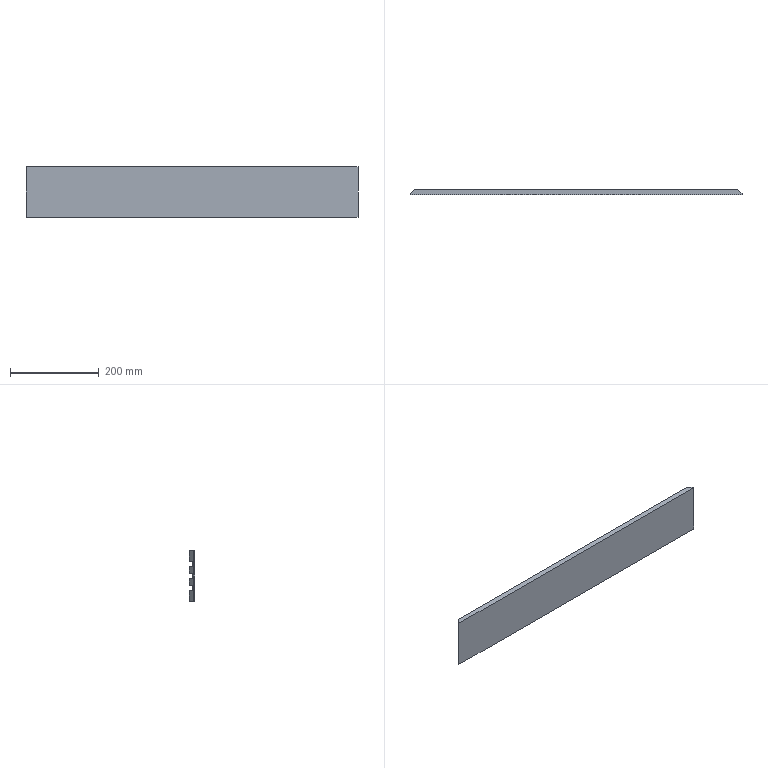Part | STEP file | 012-6-07-08 | 1 solid | 20 faces | box 750 x 12 x 114 mm | volume 828876 mm3 | plane 20
STEP:
#1=CARTESIAN_POINT('',(0.,0.,0.));
#2=DIRECTION('',(0.,0.,1.));
#3=DIRECTION('',(1.,0.,0.));
#4=AXIS2_PLACEMENT_3D('',#1,#2,#3);
#5=CARTESIAN_POINT('',(365.,6.,78.5));
#6=VERTEX_POINT('',#5);
#7=CARTESIAN_POINT('',(365.,6.,63.));
#8=VERTEX_POINT('',#7);
#9=CARTESIAN_POINT('',(365.,6.,114.));
#10=DIRECTION('',(0.,0.,-1.));
#11=VECTOR('',#10,1.);
#12=LINE('',#9,#11);
#13=CARTESIAN_POINT('',(-375.,6.,114.));
#14=DIRECTION('',(0.,-1.,0.));
#15=DIRECTION('',(0.,0.,-1.));
#16=AXIS2_PLACEMENT_3D('',#13,#14,#15);
#17=PLANE('',#16);
#18=CARTESIAN_POINT('',(0.,740.));
#19=DIRECTION('',(1.,0.));
#20=VECTOR('',#19,1.);
#21=LINE('',#18,#20);
#22=(GEOMETRIC_REPRESENTATION_CONTEXT(2)PARAMETRIC_REPRESENTATION_CONTEXT()REPRESENTATION_CONTEXT('',''));
#23=DEFINITIONAL_REPRESENTATION('',(#21),#22);
#24=PCURVE('',#17,#23);
#25=CARTESIAN_POINT('',(365.,6.,114.));
#26=DIRECTION('',(-0.7071,-0.7071,0.));
#27=DIRECTION('',(0.7071,-0.7071,0.));
#28=AXIS2_PLACEMENT_3D('',#25,#26,#27);
#29=PLANE('',#28);
#30=CARTESIAN_POINT('',(0.,0.));
#31=DIRECTION('',(0.,-1.));
#32=VECTOR('',#31,1.);
#33=LINE('',#30,#32);
#34=(GEOMETRIC_REPRESENTATION_CONTEXT(2)PARAMETRIC_REPRESENTATION_CONTEXT()REPRESENTATION_CONTEXT('',''));
#35=DEFINITIONAL_REPRESENTATION('',(#33),#34);
#36=PCURVE('',#29,#35);
#37=SURFACE_CURVE('',#12,(#24,#36),.PCURVE_S1.);
#38=EDGE_CURVE('',#6,#8,#37,.T.);
#39=ORIENTED_EDGE('',*,*,#38,.T.);
#40=CARTESIAN_POINT('',(-365.,6.,63.));
#41=VERTEX_POINT('',#40);
#42=CARTESIAN_POINT('',(378.993,6.,63.));
#43=DIRECTION('',(1.,0.,0.));
#44=VECTOR('',#43,1.);
#45=LINE('',#42,#44);
#46=CARTESIAN_POINT('',(51.,753.993));
#47=DIRECTION('',(0.,1.));
#48=VECTOR('',#47,1.);
#49=LINE('',#46,#48);
#50=(GEOMETRIC_REPRESENTATION_CONTEXT(2)PARAMETRIC_REPRESENTATION_CONTEXT()REPRESENTATION_CONTEXT('',''));
#51=DEFINITIONAL_REPRESENTATION('',(#49),#50);
#52=PCURVE('',#17,#51);
#53=CARTESIAN_POINT('',(378.993,-1.,63.));
#54=DIRECTION('',(0.,0.,1.));
#55=DIRECTION('',(1.,0.,0.));
#56=AXIS2_PLACEMENT_3D('',#53,#54,#55);
#57=PLANE('',#56);
#58=CARTESIAN_POINT('',(0.,7.));
#59=DIRECTION('',(1.,0.));
#60=VECTOR('',#59,1.);
#61=LINE('',#58,#60);
#62=(GEOMETRIC_REPRESENTATION_CONTEXT(2)PARAMETRIC_REPRESENTATION_CONTEXT()REPRESENTATION_CONTEXT('',''));
#63=DEFINITIONAL_REPRESENTATION('',(#61),#62);
#64=PCURVE('',#57,#63);
#65=SURFACE_CURVE('',#45,(#52,#64),.PCURVE_S1.);
#66=EDGE_CURVE('',#41,#8,#65,.T.);
#67=ORIENTED_EDGE('',*,*,#66,.F.);
#68=CARTESIAN_POINT('',(-365.,6.,78.5));
#69=VERTEX_POINT('',#68);
#70=CARTESIAN_POINT('',(-365.,6.,114.));
#71=DIRECTION('',(0.,0.,1.));
#72=VECTOR('',#71,1.);
#73=LINE('',#70,#72);
#74=CARTESIAN_POINT('',(0.,10.));
#75=DIRECTION('',(-1.,0.));
#76=VECTOR('',#75,1.);
#77=LINE('',#74,#76);
#78=(GEOMETRIC_REPRESENTATION_CONTEXT(2)PARAMETRIC_REPRESENTATION_CONTEXT()REPRESENTATION_CONTEXT('',''));
#79=DEFINITIONAL_REPRESENTATION('',(#77),#78);
#80=PCURVE('',#17,#79);
#81=CARTESIAN_POINT('',(-375.,-4.,114.));
#82=DIRECTION('',(0.7071,-0.7071,0.));
#83=DIRECTION('',(0.7071,0.7071,0.));
#84=AXIS2_PLACEMENT_3D('',#81,#82,#83);
#85=PLANE('',#84);
#86=CARTESIAN_POINT('',(14.142,0.));
#87=DIRECTION('',(0.,1.));
#88=VECTOR('',#87,1.);
#89=LINE('',#86,#88);
#90=(GEOMETRIC_REPRESENTATION_CONTEXT(2)PARAMETRIC_REPRESENTATION_CONTEXT()REPRESENTATION_CONTEXT('',''));
#91=DEFINITIONAL_REPRESENTATION('',(#89),#90);
#92=PCURVE('',#85,#91);
#93=SURFACE_CURVE('',#73,(#80,#92),.PCURVE_S1.);
#94=EDGE_CURVE('',#41,#69,#93,.T.);
#95=ORIENTED_EDGE('',*,*,#94,.T.);
#96=CARTESIAN_POINT('',(378.993,6.,78.5));
#97=DIRECTION('',(-1.,0.,0.));
#98=VECTOR('',#97,1.);
#99=LINE('',#96,#98);
#100=CARTESIAN_POINT('',(35.5,753.993));
#101=DIRECTION('',(0.,-1.));
#102=VECTOR('',#101,1.);
#103=LINE('',#100,#102);
#104=(GEOMETRIC_REPRESENTATION_CONTEXT(2)PARAMETRIC_REPRESENTATION_CONTEXT()REPRESENTATION_CONTEXT('',''));
#105=DEFINITIONAL_REPRESENTATION('',(#103),#104);
#106=PCURVE('',#17,#105);
#107=CARTESIAN_POINT('',(378.993,-1.,78.5));
#108=DIRECTION('',(0.,0.,-1.));
#109=DIRECTION('',(-1.,0.,0.));
#110=AXIS2_PLACEMENT_3D('',#107,#108,#109);
#111=PLANE('',#110);
#112=CARTESIAN_POINT('',(0.,7.));
#113=DIRECTION('',(1.,0.));
#114=VECTOR('',#113,1.);
#115=LINE('',#112,#114);
#116=(GEOMETRIC_REPRESENTATION_CONTEXT(2)PARAMETRIC_REPRESENTATION_CONTEXT()REPRESENTATION_CONTEXT('',''));
#117=DEFINITIONAL_REPRESENTATION('',(#115),#116);
#118=PCURVE('',#111,#117);
#119=SURFACE_CURVE('',#99,(#106,#118),.PCURVE_S1.);
#120=EDGE_CURVE('',#6,#69,#119,.T.);
#121=ORIENTED_EDGE('',*,*,#120,.F.);
#122=EDGE_LOOP('',(#39,#67,#95,#121));
#123=FACE_BOUND('',#122,.T.);
#124=ADVANCED_FACE('',(#123),#17,.F.);
#125=CARTESIAN_POINT('',(365.,6.,114.));
#126=VERTEX_POINT('',#125);
#127=CARTESIAN_POINT('',(365.,6.,90.5));
#128=VERTEX_POINT('',#127);
#129=CARTESIAN_POINT('',(365.,6.,114.));
#130=DIRECTION('',(0.,0.,-1.));
#131=VECTOR('',#130,1.);
#132=LINE('',#129,#131);
#133=CARTESIAN_POINT('',(-375.,6.,114.));
#134=DIRECTION('',(0.,-1.,0.));
#135=DIRECTION('',(0.,0.,-1.));
#136=AXIS2_PLACEMENT_3D('',#133,#134,#135);
#137=PLANE('',#136);
#138=CARTESIAN_POINT('',(0.,740.));
#139=DIRECTION('',(1.,0.));
#140=VECTOR('',#139,1.);
#141=LINE('',#138,#140);
#142=(GEOMETRIC_REPRESENTATION_CONTEXT(2)PARAMETRIC_REPRESENTATION_CONTEXT()REPRESENTATION_CONTEXT('',''));
#143=DEFINITIONAL_REPRESENTATION('',(#141),#142);
#144=PCURVE('',#137,#143);
#145=CARTESIAN_POINT('',(0.,0.));
#146=DIRECTION('',(0.,-1.));
#147=VECTOR('',#146,1.);
#148=LINE('',#145,#147);
#149=(GEOMETRIC_REPRESENTATION_CONTEXT(2)PARAMETRIC_REPRESENTATION_CONTEXT()REPRESENTATION_CONTEXT('',''));
#150=DEFINITIONAL_REPRESENTATION('',(#148),#149);
#151=PCURVE('',#29,#150);
#152=SURFACE_CURVE('',#132,(#144,#151),.PCURVE_S1.);
#153=EDGE_CURVE('',#126,#128,#152,.T.);
#154=ORIENTED_EDGE('',*,*,#153,.T.);
#155=CARTESIAN_POINT('',(-365.,6.,90.5));
#156=VERTEX_POINT('',#155);
#157=CARTESIAN_POINT('',(378.993,6.,90.5));
#158=DIRECTION('',(1.,0.,0.));
#159=VECTOR('',#158,1.);
#160=LINE('',#157,#159);
#161=CARTESIAN_POINT('',(23.5,753.993));
#162=DIRECTION('',(0.,1.));
#163=VECTOR('',#162,1.);
#164=LINE('',#161,#163);
#165=(GEOMETRIC_REPRESENTATION_CONTEXT(2)PARAMETRIC_REPRESENTATION_CONTEXT()REPRESENTATION_CONTEXT('',''));
#166=DEFINITIONAL_REPRESENTATION('',(#164),#165);
#167=PCURVE('',#137,#166);
#168=CARTESIAN_POINT('',(378.993,-1.,90.5));
#169=DIRECTION('',(0.,0.,1.));
#170=DIRECTION('',(1.,0.,0.));
#171=AXIS2_PLACEMENT_3D('',#168,#169,#170);
#172=PLANE('',#171);
#173=CARTESIAN_POINT('',(0.,7.));
#174=DIRECTION('',(1.,0.));
#175=VECTOR('',#174,1.);
#176=LINE('',#173,#175);
#177=(GEOMETRIC_REPRESENTATION_CONTEXT(2)PARAMETRIC_REPRESENTATION_CONTEXT()REPRESENTATION_CONTEXT('',''));
#178=DEFINITIONAL_REPRESENTATION('',(#176),#177);
#179=PCURVE('',#172,#178);
#180=SURFACE_CURVE('',#160,(#167,#179),.PCURVE_S1.);
#181=EDGE_CURVE('',#156,#128,#180,.T.);
#182=ORIENTED_EDGE('',*,*,#181,.F.);
#183=CARTESIAN_POINT('',(-365.,6.,114.));
#184=VERTEX_POINT('',#183);
#185=CARTESIAN_POINT('',(-365.,6.,114.));
#186=DIRECTION('',(0.,0.,1.));
#187=VECTOR('',#186,1.);
#188=LINE('',#185,#187);
#189=CARTESIAN_POINT('',(0.,10.));
#190=DIRECTION('',(-1.,0.));
#191=VECTOR('',#190,1.);
#192=LINE('',#189,#191);
#193=(GEOMETRIC_REPRESENTATION_CONTEXT(2)PARAMETRIC_REPRESENTATION_CONTEXT()REPRESENTATION_CONTEXT('',''));
#194=DEFINITIONAL_REPRESENTATION('',(#192),#193);
#195=PCURVE('',#137,#194);
#196=CARTESIAN_POINT('',(14.142,0.));
#197=DIRECTION('',(0.,1.));
#198=VECTOR('',#197,1.);
#199=LINE('',#196,#198);
#200=(GEOMETRIC_REPRESENTATION_CONTEXT(2)PARAMETRIC_REPRESENTATION_CONTEXT()REPRESENTATION_CONTEXT('',''));
#201=DEFINITIONAL_REPRESENTATION('',(#199),#200);
#202=PCURVE('',#85,#201);
#203=SURFACE_CURVE('',#188,(#195,#202),.PCURVE_S1.);
#204=EDGE_CURVE('',#156,#184,#203,.T.);
#205=ORIENTED_EDGE('',*,*,#204,.T.);
#206=CARTESIAN_POINT('',(-375.,6.,114.));
#207=DIRECTION('',(-1.,0.,0.));
#208=VECTOR('',#207,1.);
#209=LINE('',#206,#208);
#210=CARTESIAN_POINT('',(0.,0.));
#211=DIRECTION('',(0.,-1.));
#212=VECTOR('',#211,1.);
#213=LINE('',#210,#212);
#214=(GEOMETRIC_REPRESENTATION_CONTEXT(2)PARAMETRIC_REPRESENTATION_CONTEXT()REPRESENTATION_CONTEXT('',''));
#215=DEFINITIONAL_REPRESENTATION('',(#213),#214);
#216=PCURVE('',#137,#215);
#217=CARTESIAN_POINT('',(375.,-6.,114.));
#218=DIRECTION('',(0.,0.,1.));
#219=DIRECTION('',(1.,0.,0.));
#220=AXIS2_PLACEMENT_3D('',#217,#218,#219);
#221=PLANE('',#220);
#222=CARTESIAN_POINT('',(-750.,12.));
#223=DIRECTION('',(-1.,0.));
#224=VECTOR('',#223,1.);
#225=LINE('',#222,#224);
#226=(GEOMETRIC_REPRESENTATION_CONTEXT(2)PARAMETRIC_REPRESENTATION_CONTEXT()REPRESENTATION_CONTEXT('',''));
#227=DEFINITIONAL_REPRESENTATION('',(#225),#226);
#228=PCURVE('',#221,#227);
#229=SURFACE_CURVE('',#209,(#216,#228),.PCURVE_S1.);
#230=EDGE_CURVE('',#126,#184,#229,.T.);
#231=ORIENTED_EDGE('',*,*,#230,.F.);
#232=EDGE_LOOP('',(#154,#182,#205,#231));
#233=FACE_BOUND('',#232,.T.);
#234=ADVANCED_FACE('',(#233),#137,.F.);
#235=CARTESIAN_POINT('',(-365.,6.,35.5));
#236=VERTEX_POINT('',#235);
#237=CARTESIAN_POINT('',(-365.,6.,51.));
#238=VERTEX_POINT('',#237);
#239=CARTESIAN_POINT('',(-365.,6.,114.));
#240=DIRECTION('',(0.,0.,1.));
#241=VECTOR('',#240,1.);
#242=LINE('',#239,#241);
#243=CARTESIAN_POINT('',(-375.,6.,114.));
#244=DIRECTION('',(0.,-1.,0.));
#245=DIRECTION('',(0.,0.,-1.));
#246=AXIS2_PLACEMENT_3D('',#243,#244,#245);
#247=PLANE('',#246);
#248=CARTESIAN_POINT('',(0.,10.));
#249=DIRECTION('',(-1.,0.));
#250=VECTOR('',#249,1.);
#251=LINE('',#248,#250);
#252=(GEOMETRIC_REPRESENTATION_CONTEXT(2)PARAMETRIC_REPRESENTATION_CONTEXT()REPRESENTATION_CONTEXT('',''));
#253=DEFINITIONAL_REPRESENTATION('',(#251),#252);
#254=PCURVE('',#247,#253);
#255=CARTESIAN_POINT('',(14.142,0.));
#256=DIRECTION('',(0.,1.));
#257=VECTOR('',#256,1.);
#258=LINE('',#255,#257);
#259=(GEOMETRIC_REPRESENTATION_CONTEXT(2)PARAMETRIC_REPRESENTATION_CONTEXT()REPRESENTATION_CONTEXT('',''));
#260=DEFINITIONAL_REPRESENTATION('',(#258),#259);
#261=PCURVE('',#85,#260);
#262=SURFACE_CURVE('',#242,(#254,#261),.PCURVE_S1.);
#263=EDGE_CURVE('',#236,#238,#262,.T.);
#264=ORIENTED_EDGE('',*,*,#263,.T.);
#265=CARTESIAN_POINT('',(365.,6.,51.));
#266=VERTEX_POINT('',#265);
#267=CARTESIAN_POINT('',(378.993,6.,51.));
#268=DIRECTION('',(-1.,0.,0.));
#269=VECTOR('',#268,1.);
#270=LINE('',#267,#269);
#271=CARTESIAN_POINT('',(63.,753.993));
#272=DIRECTION('',(0.,-1.));
#273=VECTOR('',#272,1.);
#274=LINE('',#271,#273);
#275=(GEOMETRIC_REPRESENTATION_CONTEXT(2)PARAMETRIC_REPRESENTATION_CONTEXT()REPRESENTATION_CONTEXT('',''));
#276=DEFINITIONAL_REPRESENTATION('',(#274),#275);
#277=PCURVE('',#247,#276);
#278=CARTESIAN_POINT('',(378.993,-1.,51.));
#279=DIRECTION('',(0.,0.,-1.));
#280=DIRECTION('',(-1.,0.,0.));
#281=AXIS2_PLACEMENT_3D('',#278,#279,#280);
#282=PLANE('',#281);
#283=CARTESIAN_POINT('',(0.,7.));
#284=DIRECTION('',(1.,0.));
#285=VECTOR('',#284,1.);
#286=LINE('',#283,#285);
#287=(GEOMETRIC_REPRESENTATION_CONTEXT(2)PARAMETRIC_REPRESENTATION_CONTEXT()REPRESENTATION_CONTEXT('',''));
#288=DEFINITIONAL_REPRESENTATION('',(#286),#287);
#289=PCURVE('',#282,#288);
#290=SURFACE_CURVE('',#270,(#277,#289),.PCURVE_S1.);
#291=EDGE_CURVE('',#266,#238,#290,.T.);
#292=ORIENTED_EDGE('',*,*,#291,.F.);
#293=CARTESIAN_POINT('',(365.,6.,35.5));
#294=VERTEX_POINT('',#293);
#295=CARTESIAN_POINT('',(365.,6.,114.));
#296=DIRECTION('',(0.,0.,-1.));
#297=VECTOR('',#296,1.);
#298=LINE('',#295,#297);
#299=CARTESIAN_POINT('',(0.,740.));
#300=DIRECTION('',(1.,0.));
#301=VECTOR('',#300,1.);
#302=LINE('',#299,#301);
#303=(GEOMETRIC_REPRESENTATION_CONTEXT(2)PARAMETRIC_REPRESENTATION_CONTEXT()REPRESENTATION_CONTEXT('',''));
#304=DEFINITIONAL_REPRESENTATION('',(#302),#303);
#305=PCURVE('',#247,#304);
#306=CARTESIAN_POINT('',(0.,0.));
#307=DIRECTION('',(0.,-1.));
#308=VECTOR('',#307,1.);
#309=LINE('',#306,#308);
#310=(GEOMETRIC_REPRESENTATION_CONTEXT(2)PARAMETRIC_REPRESENTATION_CONTEXT()REPRESENTATION_CONTEXT('',''));
#311=DEFINITIONAL_REPRESENTATION('',(#309),#310);
#312=PCURVE('',#29,#311);
#313=SURFACE_CURVE('',#298,(#305,#312),.PCURVE_S1.);
#314=EDGE_CURVE('',#266,#294,#313,.T.);
#315=ORIENTED_EDGE('',*,*,#314,.T.);
#316=CARTESIAN_POINT('',(378.993,6.,35.5));
#317=DIRECTION('',(1.,0.,0.));
#318=VECTOR('',#317,1.);
#319=LINE('',#316,#318);
#320=CARTESIAN_POINT('',(78.5,753.993));
#321=DIRECTION('',(0.,1.));
#322=VECTOR('',#321,1.);
#323=LINE('',#320,#322);
#324=(GEOMETRIC_REPRESENTATION_CONTEXT(2)PARAMETRIC_REPRESENTATION_CONTEXT()REPRESENTATION_CONTEXT('',''));
#325=DEFINITIONAL_REPRESENTATION('',(#323),#324);
#326=PCURVE('',#247,#325);
#327=CARTESIAN_POINT('',(378.993,-1.,35.5));
#328=DIRECTION('',(0.,0.,1.));
#329=DIRECTION('',(1.,0.,0.));
#330=AXIS2_PLACEMENT_3D('',#327,#328,#329);
#331=PLANE('',#330);
#332=CARTESIAN_POINT('',(0.,7.));
#333=DIRECTION('',(1.,0.));
#334=VECTOR('',#333,1.);
#335=LINE('',#332,#334);
#336=(GEOMETRIC_REPRESENTATION_CONTEXT(2)PARAMETRIC_REPRESENTATION_CONTEXT()REPRESENTATION_CONTEXT('',''));
#337=DEFINITIONAL_REPRESENTATION('',(#335),#336);
#338=PCURVE('',#331,#337);
#339=SURFACE_CURVE('',#319,(#326,#338),.PCURVE_S1.);
#340=EDGE_CURVE('',#236,#294,#339,.T.);
#341=ORIENTED_EDGE('',*,*,#340,.F.);
#342=EDGE_LOOP('',(#264,#292,#315,#341));
#343=FACE_BOUND('',#342,.T.);
#344=ADVANCED_FACE('',(#343),#247,.F.);
#345=CARTESIAN_POINT('',(375.,-6.,0.));
#346=VERTEX_POINT('',#345);
#347=CARTESIAN_POINT('',(375.,-4.,0.));
#348=VERTEX_POINT('',#347);
#349=CARTESIAN_POINT('',(375.,6.,0.));
#350=DIRECTION('',(0.,1.,0.));
#351=VECTOR('',#350,1.);
#352=LINE('',#349,#351);
#353=CARTESIAN_POINT('',(375.,6.,114.));
#354=DIRECTION('',(-1.,0.,0.));
#355=DIRECTION('',(0.,0.,1.));
#356=AXIS2_PLACEMENT_3D('',#353,#354,#355);
#357=PLANE('',#356);
#358=CARTESIAN_POINT('',(-114.,0.));
#359=DIRECTION('',(0.,1.));
#360=VECTOR('',#359,1.);
#361=LINE('',#358,#360);
#362=(GEOMETRIC_REPRESENTATION_CONTEXT(2)PARAMETRIC_REPRESENTATION_CONTEXT()REPRESENTATION_CONTEXT('',''));
#363=DEFINITIONAL_REPRESENTATION('',(#361),#362);
#364=PCURVE('',#357,#363);
#365=CARTESIAN_POINT('',(375.,-6.,0.));
#366=DIRECTION('',(0.,0.,1.));
#367=DIRECTION('',(1.,0.,0.));
#368=AXIS2_PLACEMENT_3D('',#365,#366,#367);
#369=PLANE('',#368);
#370=CARTESIAN_POINT('',(0.,12.));
#371=DIRECTION('',(0.,1.));
#372=VECTOR('',#371,1.);
#373=LINE('',#370,#372);
#374=(GEOMETRIC_REPRESENTATION_CONTEXT(2)PARAMETRIC_REPRESENTATION_CONTEXT()REPRESENTATION_CONTEXT('',''));
#375=DEFINITIONAL_REPRESENTATION('',(#373),#374);
#376=PCURVE('',#369,#375);
#377=SURFACE_CURVE('',#352,(#364,#376),.PCURVE_S1.);
#378=EDGE_CURVE('',#346,#348,#377,.T.);
#379=ORIENTED_EDGE('',*,*,#378,.T.);
#380=CARTESIAN_POINT('',(375.,-4.,114.));
#381=VERTEX_POINT('',#380);
#382=CARTESIAN_POINT('',(375.,-4.,114.));
#383=DIRECTION('',(0.,0.,1.));
#384=VECTOR('',#383,1.);
#385=LINE('',#382,#384);
#386=CARTESIAN_POINT('',(0.,-10.));
#387=DIRECTION('',(1.,0.));
#388=VECTOR('',#387,1.);
#389=LINE('',#386,#388);
#390=(GEOMETRIC_REPRESENTATION_CONTEXT(2)PARAMETRIC_REPRESENTATION_CONTEXT()REPRESENTATION_CONTEXT('',''));
#391=DEFINITIONAL_REPRESENTATION('',(#389),#390);
#392=PCURVE('',#357,#391);
#393=CARTESIAN_POINT('',(14.142,0.));
#394=DIRECTION('',(0.,1.));
#395=VECTOR('',#394,1.);
#396=LINE('',#393,#395);
#397=(GEOMETRIC_REPRESENTATION_CONTEXT(2)PARAMETRIC_REPRESENTATION_CONTEXT()REPRESENTATION_CONTEXT('',''));
#398=DEFINITIONAL_REPRESENTATION('',(#396),#397);
#399=PCURVE('',#29,#398);
#400=SURFACE_CURVE('',#385,(#392,#399),.PCURVE_S1.);
#401=EDGE_CURVE('',#348,#381,#400,.T.);
#402=ORIENTED_EDGE('',*,*,#401,.T.);
#403=CARTESIAN_POINT('',(375.,-6.,114.));
#404=VERTEX_POINT('',#403);
#405=CARTESIAN_POINT('',(375.,6.,114.));
#406=DIRECTION('',(0.,1.,0.));
#407=VECTOR('',#406,1.);
#408=LINE('',#405,#407);
#409=CARTESIAN_POINT('',(0.,0.));
#410=DIRECTION('',(0.,1.));
#411=VECTOR('',#410,1.);
#412=LINE('',#409,#411);
#413=(GEOMETRIC_REPRESENTATION_CONTEXT(2)PARAMETRIC_REPRESENTATION_CONTEXT()REPRESENTATION_CONTEXT('',''));
#414=DEFINITIONAL_REPRESENTATION('',(#412),#413);
#415=PCURVE('',#357,#414);
#416=CARTESIAN_POINT('',(0.,12.));
#417=DIRECTION('',(0.,1.));
#418=VECTOR('',#417,1.);
#419=LINE('',#416,#418);
#420=(GEOMETRIC_REPRESENTATION_CONTEXT(2)PARAMETRIC_REPRESENTATION_CONTEXT()REPRESENTATION_CONTEXT('',''));
#421=DEFINITIONAL_REPRESENTATION('',(#419),#420);
#422=PCURVE('',#221,#421);
#423=SURFACE_CURVE('',#408,(#415,#422),.PCURVE_S1.);
#424=EDGE_CURVE('',#404,#381,#423,.T.);
#425=ORIENTED_EDGE('',*,*,#424,.F.);
#426=CARTESIAN_POINT('',(375.,-6.,114.));
#427=DIRECTION('',(0.,0.,-1.));
#428=VECTOR('',#427,1.);
#429=LINE('',#426,#428);
#430=CARTESIAN_POINT('',(0.,-12.));
#431=DIRECTION('',(-1.,0.));
#432=VECTOR('',#431,1.);
#433=LINE('',#430,#432);
#434=(GEOMETRIC_REPRESENTATION_CONTEXT(2)PARAMETRIC_REPRESENTATION_CONTEXT()REPRESENTATION_CONTEXT('',''));
#435=DEFINITIONAL_REPRESENTATION('',(#433),#434);
#436=PCURVE('',#357,#435);
#437=CARTESIAN_POINT('',(-375.,-6.,114.));
#438=DIRECTION('',(0.,1.,0.));
#439=DIRECTION('',(0.,0.,1.));
#440=AXIS2_PLACEMENT_3D('',#437,#438,#439);
#441=PLANE('',#440);
#442=CARTESIAN_POINT('',(0.,750.));
#443=DIRECTION('',(-1.,0.));
#444=VECTOR('',#443,1.);
#445=LINE('',#442,#444);
#446=(GEOMETRIC_REPRESENTATION_CONTEXT(2)PARAMETRIC_REPRESENTATION_CONTEXT()REPRESENTATION_CONTEXT('',''));
#447=DEFINITIONAL_REPRESENTATION('',(#445),#446);
#448=PCURVE('',#441,#447);
#449=SURFACE_CURVE('',#429,(#436,#448),.PCURVE_S1.);
#450=EDGE_CURVE('',#404,#346,#449,.T.);
#451=ORIENTED_EDGE('',*,*,#450,.T.);
#452=EDGE_LOOP('',(#379,#402,#425,#451));
#453=FACE_BOUND('',#452,.T.);
#454=ADVANCED_FACE('',(#453),#357,.F.);
#455=CARTESIAN_POINT('',(-365.,6.,0.));
#456=VERTEX_POINT('',#455);
#457=CARTESIAN_POINT('',(-365.,6.,23.5));
#458=VERTEX_POINT('',#457);
#459=CARTESIAN_POINT('',(-365.,6.,114.));
#460=DIRECTION('',(0.,0.,1.));
#461=VECTOR('',#460,1.);
#462=LINE('',#459,#461);
#463=CARTESIAN_POINT('',(-375.,6.,114.));
#464=DIRECTION('',(0.,-1.,0.));
#465=DIRECTION('',(0.,0.,-1.));
#466=AXIS2_PLACEMENT_3D('',#463,#464,#465);
#467=PLANE('',#466);
#468=CARTESIAN_POINT('',(0.,10.));
#469=DIRECTION('',(-1.,0.));
#470=VECTOR('',#469,1.);
#471=LINE('',#468,#470);
#472=(GEOMETRIC_REPRESENTATION_CONTEXT(2)PARAMETRIC_REPRESENTATION_CONTEXT()REPRESENTATION_CONTEXT('',''));
#473=DEFINITIONAL_REPRESENTATION('',(#471),#472);
#474=PCURVE('',#467,#473);
#475=CARTESIAN_POINT('',(14.142,0.));
#476=DIRECTION('',(0.,1.));
#477=VECTOR('',#476,1.);
#478=LINE('',#475,#477);
#479=(GEOMETRIC_REPRESENTATION_CONTEXT(2)PARAMETRIC_REPRESENTATION_CONTEXT()REPRESENTATION_CONTEXT('',''));
#480=DEFINITIONAL_REPRESENTATION('',(#478),#479);
#481=PCURVE('',#85,#480);
#482=SURFACE_CURVE('',#462,(#474,#481),.PCURVE_S1.);
#483=EDGE_CURVE('',#456,#458,#482,.T.);
#484=ORIENTED_EDGE('',*,*,#483,.T.);
#485=CARTESIAN_POINT('',(365.,6.,23.5));
#486=VERTEX_POINT('',#485);
#487=CARTESIAN_POINT('',(378.993,6.,23.5));
#488=DIRECTION('',(-1.,0.,0.));
#489=VECTOR('',#488,1.);
#490=LINE('',#487,#489);
#491=CARTESIAN_POINT('',(90.5,753.993));
#492=DIRECTION('',(0.,-1.));
#493=VECTOR('',#492,1.);
#494=LINE('',#491,#493);
#495=(GEOMETRIC_REPRESENTATION_CONTEXT(2)PARAMETRIC_REPRESENTATION_CONTEXT()REPRESENTATION_CONTEXT('',''));
#496=DEFINITIONAL_REPRESENTATION('',(#494),#495);
#497=PCURVE('',#467,#496);
#498=CARTESIAN_POINT('',(378.993,-1.,23.5));
#499=DIRECTION('',(0.,0.,-1.));
#500=DIRECTION('',(-1.,0.,0.));
#501=AXIS2_PLACEMENT_3D('',#498,#499,#500);
#502=PLANE('',#501);
#503=CARTESIAN_POINT('',(0.,7.));
#504=DIRECTION('',(1.,0.));
#505=VECTOR('',#504,1.);
#506=LINE('',#503,#505);
#507=(GEOMETRIC_REPRESENTATION_CONTEXT(2)PARAMETRIC_REPRESENTATION_CONTEXT()REPRESENTATION_CONTEXT('',''));
#508=DEFINITIONAL_REPRESENTATION('',(#506),#507);
#509=PCURVE('',#502,#508);
#510=SURFACE_CURVE('',#490,(#497,#509),.PCURVE_S1.);
#511=EDGE_CURVE('',#486,#458,#510,.T.);
#512=ORIENTED_EDGE('',*,*,#511,.F.);
#513=CARTESIAN_POINT('',(365.,6.,0.));
#514=VERTEX_POINT('',#513);
#515=CARTESIAN_POINT('',(365.,6.,114.));
#516=DIRECTION('',(0.,0.,-1.));
#517=VECTOR('',#516,1.);
#518=LINE('',#515,#517);
#519=CARTESIAN_POINT('',(0.,740.));
#520=DIRECTION('',(1.,0.));
#521=VECTOR('',#520,1.);
#522=LINE('',#519,#521);
#523=(GEOMETRIC_REPRESENTATION_CONTEXT(2)PARAMETRIC_REPRESENTATION_CONTEXT()REPRESENTATION_CONTEXT('',''));
#524=DEFINITIONAL_REPRESENTATION('',(#522),#523);
#525=PCURVE('',#467,#524);
#526=CARTESIAN_POINT('',(0.,0.));
#527=DIRECTION('',(0.,-1.));
#528=VECTOR('',#527,1.);
#529=LINE('',#526,#528);
#530=(GEOMETRIC_REPRESENTATION_CONTEXT(2)PARAMETRIC_REPRESENTATION_CONTEXT()REPRESENTATION_CONTEXT('',''));
#531=DEFINITIONAL_REPRESENTATION('',(#529),#530);
#532=PCURVE('',#29,#531);
#533=SURFACE_CURVE('',#518,(#525,#532),.PCURVE_S1.);
#534=EDGE_CURVE('',#486,#514,#533,.T.);
#535=ORIENTED_EDGE('',*,*,#534,.T.);
#536=CARTESIAN_POINT('',(-375.,6.,0.));
#537=DIRECTION('',(-1.,0.,0.));
#538=VECTOR('',#537,1.);
#539=LINE('',#536,#538);
#540=CARTESIAN_POINT('',(114.,0.));
#541=DIRECTION('',(0.,-1.));
#542=VECTOR('',#541,1.);
#543=LINE('',#540,#542);
#544=(GEOMETRIC_REPRESENTATION_CONTEXT(2)PARAMETRIC_REPRESENTATION_CONTEXT()REPRESENTATION_CONTEXT('',''));
#545=DEFINITIONAL_REPRESENTATION('',(#543),#544);
#546=PCURVE('',#467,#545);
#547=CARTESIAN_POINT('',(-750.,12.));
#548=DIRECTION('',(-1.,0.));
#549=VECTOR('',#548,1.);
#550=LINE('',#547,#549);
#551=(GEOMETRIC_REPRESENTATION_CONTEXT(2)PARAMETRIC_REPRESENTATION_CONTEXT()REPRESENTATION_CONTEXT('',''));
#552=DEFINITIONAL_REPRESENTATION('',(#550),#551);
#553=PCURVE('',#369,#552);
#554=SURFACE_CURVE('',#539,(#546,#553),.PCURVE_S1.);
#555=EDGE_CURVE('',#514,#456,#554,.T.);
#556=ORIENTED_EDGE('',*,*,#555,.T.);
#557=EDGE_LOOP('',(#484,#512,#535,#556));
#558=FACE_BOUND('',#557,.T.);
#559=ADVANCED_FACE('',(#558),#467,.F.);
#560=CARTESIAN_POINT('',(-375.,-4.,114.));
#561=VERTEX_POINT('',#560);
#562=CARTESIAN_POINT('',(-375.,-6.,114.));
#563=VERTEX_POINT('',#562);
#564=CARTESIAN_POINT('',(-375.,6.,114.));
#565=DIRECTION('',(0.,-1.,0.));
#566=VECTOR('',#565,1.);
#567=LINE('',#564,#566);
#568=CARTESIAN_POINT('',(-375.,6.,114.));
#569=DIRECTION('',(1.,0.,0.));
#570=DIRECTION('',(0.,0.,-1.));
#571=AXIS2_PLACEMENT_3D('',#568,#569,#570);
#572=PLANE('',#571);
#573=CARTESIAN_POINT('',(0.,0.));
#574=DIRECTION('',(0.,-1.));
#575=VECTOR('',#574,1.);
#576=LINE('',#573,#575);
#577=(GEOMETRIC_REPRESENTATION_CONTEXT(2)PARAMETRIC_REPRESENTATION_CONTEXT()REPRESENTATION_CONTEXT('',''));
#578=DEFINITIONAL_REPRESENTATION('',(#576),#577);
#579=PCURVE('',#572,#578);
#580=CARTESIAN_POINT('',(-750.,12.));
#581=DIRECTION('',(0.,-1.));
#582=VECTOR('',#581,1.);
#583=LINE('',#580,#582);
#584=(GEOMETRIC_REPRESENTATION_CONTEXT(2)PARAMETRIC_REPRESENTATION_CONTEXT()REPRESENTATION_CONTEXT('',''));
#585=DEFINITIONAL_REPRESENTATION('',(#583),#584);
#586=PCURVE('',#221,#585);
#587=SURFACE_CURVE('',#567,(#579,#586),.PCURVE_S1.);
#588=EDGE_CURVE('',#561,#563,#587,.T.);
#589=ORIENTED_EDGE('',*,*,#588,.F.);
#590=CARTESIAN_POINT('',(-375.,-4.,0.));
#591=VERTEX_POINT('',#590);
#592=CARTESIAN_POINT('',(-375.,-4.,114.));
#593=DIRECTION('',(0.,0.,-1.));
#594=VECTOR('',#593,1.);
#595=LINE('',#592,#594);
#596=CARTESIAN_POINT('',(0.,-10.));
#597=DIRECTION('',(1.,0.));
#598=VECTOR('',#597,1.);
#599=LINE('',#596,#598);
#600=(GEOMETRIC_REPRESENTATION_CONTEXT(2)PARAMETRIC_REPRESENTATION_CONTEXT()REPRESENTATION_CONTEXT('',''));
#601=DEFINITIONAL_REPRESENTATION('',(#599),#600);
#602=PCURVE('',#572,#601);
#603=CARTESIAN_POINT('',(0.,0.));
#604=DIRECTION('',(0.,-1.));
#605=VECTOR('',#604,1.);
#606=LINE('',#603,#605);
#607=(GEOMETRIC_REPRESENTATION_CONTEXT(2)PARAMETRIC_REPRESENTATION_CONTEXT()REPRESENTATION_CONTEXT('',''));
#608=DEFINITIONAL_REPRESENTATION('',(#606),#607);
#609=PCURVE('',#85,#608);
#610=SURFACE_CURVE('',#595,(#602,#609),.PCURVE_S1.);
#611=EDGE_CURVE('',#561,#591,#610,.T.);
#612=ORIENTED_EDGE('',*,*,#611,.T.);
#613=CARTESIAN_POINT('',(-375.,-6.,0.));
#614=VERTEX_POINT('',#613);
#615=CARTESIAN_POINT('',(-375.,6.,0.));
#616=DIRECTION('',(0.,-1.,0.));
#617=VECTOR('',#616,1.);
#618=LINE('',#615,#617);
#619=CARTESIAN_POINT('',(114.,0.));
#620=DIRECTION('',(0.,-1.));
#621=VECTOR('',#620,1.);
#622=LINE('',#619,#621);
#623=(GEOMETRIC_REPRESENTATION_CONTEXT(2)PARAMETRIC_REPRESENTATION_CONTEXT()REPRESENTATION_CONTEXT('',''));
#624=DEFINITIONAL_REPRESENTATION('',(#622),#623);
#625=PCURVE('',#572,#624);
#626=CARTESIAN_POINT('',(-750.,12.));
#627=DIRECTION('',(0.,-1.));
#628=VECTOR('',#627,1.);
#629=LINE('',#626,#628);
#630=(GEOMETRIC_REPRESENTATION_CONTEXT(2)PARAMETRIC_REPRESENTATION_CONTEXT()REPRESENTATION_CONTEXT('',''));
#631=DEFINITIONAL_REPRESENTATION('',(#629),#630);
#632=PCURVE('',#369,#631);
#633=SURFACE_CURVE('',#618,(#625,#632),.PCURVE_S1.);
#634=EDGE_CURVE('',#591,#614,#633,.T.);
#635=ORIENTED_EDGE('',*,*,#634,.T.);
#636=CARTESIAN_POINT('',(-375.,-6.,114.));
#637=DIRECTION('',(0.,0.,-1.));
#638=VECTOR('',#637,1.);
#639=LINE('',#636,#638);
#640=CARTESIAN_POINT('',(0.,-12.));
#641=DIRECTION('',(1.,0.));
#642=VECTOR('',#641,1.);
#643=LINE('',#640,#642);
#644=(GEOMETRIC_REPRESENTATION_CONTEXT(2)PARAMETRIC_REPRESENTATION_CONTEXT()REPRESENTATION_CONTEXT('',''));
#645=DEFINITIONAL_REPRESENTATION('',(#643),#644);
#646=PCURVE('',#572,#645);
#647=CARTESIAN_POINT('',(0.,0.));
#648=DIRECTION('',(-1.,0.));
#649=VECTOR('',#648,1.);
#650=LINE('',#647,#649);
#651=(GEOMETRIC_REPRESENTATION_CONTEXT(2)PARAMETRIC_REPRESENTATION_CONTEXT()REPRESENTATION_CONTEXT('',''));
#652=DEFINITIONAL_REPRESENTATION('',(#650),#651);
#653=PCURVE('',#441,#652);
#654=SURFACE_CURVE('',#639,(#646,#653),.PCURVE_S1.);
#655=EDGE_CURVE('',#563,#614,#654,.T.);
#656=ORIENTED_EDGE('',*,*,#655,.F.);
#657=EDGE_LOOP('',(#589,#612,#635,#656));
#658=FACE_BOUND('',#657,.T.);
#659=ADVANCED_FACE('',(#658),#572,.F.);
#660=CARTESIAN_POINT('',(-375.,-6.,0.));
#661=DIRECTION('',(1.,0.,0.));
#662=VECTOR('',#661,1.);
#663=LINE('',#660,#662);
#664=CARTESIAN_POINT('',(-114.,0.));
#665=DIRECTION('',(0.,1.));
#666=VECTOR('',#665,1.);
#667=LINE('',#664,#666);
#668=(GEOMETRIC_REPRESENTATION_CONTEXT(2)PARAMETRIC_REPRESENTATION_CONTEXT()REPRESENTATION_CONTEXT('',''));
#669=DEFINITIONAL_REPRESENTATION('',(#667),#668);
#670=PCURVE('',#441,#669);
#671=CARTESIAN_POINT('',(-750.,0.));
#672=DIRECTION('',(1.,0.));
#673=VECTOR('',#672,1.);
#674=LINE('',#671,#673);
#675=(GEOMETRIC_REPRESENTATION_CONTEXT(2)PARAMETRIC_REPRESENTATION_CONTEXT()REPRESENTATION_CONTEXT('',''));
#676=DEFINITIONAL_REPRESENTATION('',(#674),#675);
#677=PCURVE('',#369,#676);
#678=SURFACE_CURVE('',#663,(#670,#677),.PCURVE_S1.);
#679=EDGE_CURVE('',#614,#346,#678,.T.);
#680=ORIENTED_EDGE('',*,*,#679,.T.);
#681=ORIENTED_EDGE('',*,*,#450,.F.);
#682=CARTESIAN_POINT('',(-375.,-6.,114.));
#683=DIRECTION('',(1.,0.,0.));
#684=VECTOR('',#683,1.);
#685=LINE('',#682,#684);
#686=CARTESIAN_POINT('',(0.,0.));
#687=DIRECTION('',(0.,1.));
#688=VECTOR('',#687,1.);
#689=LINE('',#686,#688);
#690=(GEOMETRIC_REPRESENTATION_CONTEXT(2)PARAMETRIC_REPRESENTATION_CONTEXT()REPRESENTATION_CONTEXT('',''));
#691=DEFINITIONAL_REPRESENTATION('',(#689),#690);
#692=PCURVE('',#441,#691);
#693=CARTESIAN_POINT('',(-750.,0.));
#694=DIRECTION('',(1.,0.));
#695=VECTOR('',#694,1.);
#696=LINE('',#693,#695);
#697=(GEOMETRIC_REPRESENTATION_CONTEXT(2)PARAMETRIC_REPRESENTATION_CONTEXT()REPRESENTATION_CONTEXT('',''));
#698=DEFINITIONAL_REPRESENTATION('',(#696),#697);
#699=PCURVE('',#221,#698);
#700=SURFACE_CURVE('',#685,(#692,#699),.PCURVE_S1.);
#701=EDGE_CURVE('',#563,#404,#700,.T.);
#702=ORIENTED_EDGE('',*,*,#701,.F.);
#703=ORIENTED_EDGE('',*,*,#655,.T.);
#704=EDGE_LOOP('',(#680,#681,#702,#703));
#705=FACE_BOUND('',#704,.T.);
#706=ADVANCED_FACE('',(#705),#441,.F.);
#707=ORIENTED_EDGE('',*,*,#424,.T.);
#708=CARTESIAN_POINT('',(376.,-5.,114.));
#709=DIRECTION('',(-0.7071,0.7071,0.));
#710=VECTOR('',#709,1.);
#711=LINE('',#708,#710);
#712=CARTESIAN_POINT('',(1.,1.));
#713=DIRECTION('',(-0.7071,0.7071));
#714=VECTOR('',#713,1.);
#715=LINE('',#712,#714);
#716=(GEOMETRIC_REPRESENTATION_CONTEXT(2)PARAMETRIC_REPRESENTATION_CONTEXT()REPRESENTATION_CONTEXT('',''));
#717=DEFINITIONAL_REPRESENTATION('',(#715),#716);
#718=PCURVE('',#221,#717);
#719=CARTESIAN_POINT('',(15.556,0.));
#720=DIRECTION('',(-1.,0.));
#721=VECTOR('',#720,1.);
#722=LINE('',#719,#721);
#723=(GEOMETRIC_REPRESENTATION_CONTEXT(2)PARAMETRIC_REPRESENTATION_CONTEXT()REPRESENTATION_CONTEXT('',''));
#724=DEFINITIONAL_REPRESENTATION('',(#722),#723);
#725=PCURVE('',#29,#724);
#726=SURFACE_CURVE('',#711,(#718,#725),.PCURVE_S1.);
#727=EDGE_CURVE('',#381,#126,#726,.T.);
#728=ORIENTED_EDGE('',*,*,#727,.T.);
#729=ORIENTED_EDGE('',*,*,#230,.T.);
#730=CARTESIAN_POINT('',(-1.,370.,114.));
#731=DIRECTION('',(-0.7071,-0.7071,0.));
#732=VECTOR('',#731,1.);
#733=LINE('',#730,#732);
#734=CARTESIAN_POINT('',(-376.,376.));
#735=DIRECTION('',(-0.7071,-0.7071));
#736=VECTOR('',#735,1.);
#737=LINE('',#734,#736);
#738=(GEOMETRIC_REPRESENTATION_CONTEXT(2)PARAMETRIC_REPRESENTATION_CONTEXT()REPRESENTATION_CONTEXT('',''));
#739=DEFINITIONAL_REPRESENTATION('',(#737),#738);
#740=PCURVE('',#221,#739);
#741=CARTESIAN_POINT('',(528.916,0.));
#742=DIRECTION('',(-1.,0.));
#743=VECTOR('',#742,1.);
#744=LINE('',#741,#743);
#745=(GEOMETRIC_REPRESENTATION_CONTEXT(2)PARAMETRIC_REPRESENTATION_CONTEXT()REPRESENTATION_CONTEXT('',''));
#746=DEFINITIONAL_REPRESENTATION('',(#744),#745);
#747=PCURVE('',#85,#746);
#748=SURFACE_CURVE('',#733,(#740,#747),.PCURVE_S1.);
#749=EDGE_CURVE('',#184,#561,#748,.T.);
#750=ORIENTED_EDGE('',*,*,#749,.T.);
#751=ORIENTED_EDGE('',*,*,#588,.T.);
#752=ORIENTED_EDGE('',*,*,#701,.T.);
#753=EDGE_LOOP('',(#707,#728,#729,#750,#751,#752));
#754=FACE_BOUND('',#753,.T.);
#755=ADVANCED_FACE('',(#754),#221,.T.);
#756=ORIENTED_EDGE('',*,*,#555,.F.);
#757=CARTESIAN_POINT('',(365.,6.,0.));
#758=DIRECTION('',(0.7071,-0.7071,0.));
#759=VECTOR('',#758,1.);
#760=LINE('',#757,#759);
#761=CARTESIAN_POINT('',(-10.,12.));
#762=DIRECTION('',(0.7071,-0.7071));
#763=VECTOR('',#762,1.);
#764=LINE('',#761,#763);
#765=(GEOMETRIC_REPRESENTATION_CONTEXT(2)PARAMETRIC_REPRESENTATION_CONTEXT()REPRESENTATION_CONTEXT('',''));
#766=DEFINITIONAL_REPRESENTATION('',(#764),#765);
#767=PCURVE('',#369,#766);
#768=CARTESIAN_POINT('',(0.,-114.));
#769=DIRECTION('',(1.,0.));
#770=VECTOR('',#769,1.);
#771=LINE('',#768,#770);
#772=(GEOMETRIC_REPRESENTATION_CONTEXT(2)PARAMETRIC_REPRESENTATION_CONTEXT()REPRESENTATION_CONTEXT('',''));
#773=DEFINITIONAL_REPRESENTATION('',(#771),#772);
#774=PCURVE('',#29,#773);
#775=SURFACE_CURVE('',#760,(#767,#774),.PCURVE_S1.);
#776=EDGE_CURVE('',#514,#348,#775,.T.);
#777=ORIENTED_EDGE('',*,*,#776,.T.);
#778=ORIENTED_EDGE('',*,*,#378,.F.);
#779=ORIENTED_EDGE('',*,*,#679,.F.);
#780=ORIENTED_EDGE('',*,*,#634,.F.);
#781=CARTESIAN_POINT('',(-375.,-4.,0.));
#782=DIRECTION('',(0.7071,0.7071,0.));
#783=VECTOR('',#782,1.);
#784=LINE('',#781,#783);
#785=CARTESIAN_POINT('',(-750.,2.));
#786=DIRECTION('',(0.7071,0.7071));
#787=VECTOR('',#786,1.);
#788=LINE('',#785,#787);
#789=(GEOMETRIC_REPRESENTATION_CONTEXT(2)PARAMETRIC_REPRESENTATION_CONTEXT()REPRESENTATION_CONTEXT('',''));
#790=DEFINITIONAL_REPRESENTATION('',(#788),#789);
#791=PCURVE('',#369,#790);
#792=CARTESIAN_POINT('',(0.,-114.));
#793=DIRECTION('',(1.,0.));
#794=VECTOR('',#793,1.);
#795=LINE('',#792,#794);
#796=(GEOMETRIC_REPRESENTATION_CONTEXT(2)PARAMETRIC_REPRESENTATION_CONTEXT()REPRESENTATION_CONTEXT('',''));
#797=DEFINITIONAL_REPRESENTATION('',(#795),#796);
#798=PCURVE('',#85,#797);
#799=SURFACE_CURVE('',#784,(#791,#798),.PCURVE_S1.);
#800=EDGE_CURVE('',#591,#456,#799,.T.);
#801=ORIENTED_EDGE('',*,*,#800,.T.);
#802=EDGE_LOOP('',(#756,#777,#778,#779,#780,#801));
#803=FACE_BOUND('',#802,.T.);
#804=ADVANCED_FACE('',(#803),#369,.F.);
#805=CARTESIAN_POINT('',(372.,-1.,63.));
#806=VERTEX_POINT('',#805);
#807=CARTESIAN_POINT('',(365.,6.,63.));
#808=DIRECTION('',(0.7071,-0.7071,0.));
#809=VECTOR('',#808,1.);
#810=LINE('',#807,#809);
#811=CARTESIAN_POINT('',(0.,-51.));
#812=DIRECTION('',(1.,0.));
#813=VECTOR('',#812,1.);
#814=LINE('',#811,#813);
#815=(GEOMETRIC_REPRESENTATION_CONTEXT(2)PARAMETRIC_REPRESENTATION_CONTEXT()REPRESENTATION_CONTEXT('',''));
#816=DEFINITIONAL_REPRESENTATION('',(#814),#815);
#817=PCURVE('',#29,#816);
#818=CARTESIAN_POINT('',(-13.993,7.));
#819=DIRECTION('',(0.7071,-0.7071));
#820=VECTOR('',#819,1.);
#821=LINE('',#818,#820);
#822=(GEOMETRIC_REPRESENTATION_CONTEXT(2)PARAMETRIC_REPRESENTATION_CONTEXT()REPRESENTATION_CONTEXT('',''));
#823=DEFINITIONAL_REPRESENTATION('',(#821),#822);
#824=PCURVE('',#57,#823);
#825=SURFACE_CURVE('',#810,(#817,#824),.PCURVE_S1.);
#826=EDGE_CURVE('',#8,#806,#825,.T.);
#827=ORIENTED_EDGE('',*,*,#826,.F.);
#828=ORIENTED_EDGE('',*,*,#38,.F.);
#829=CARTESIAN_POINT('',(372.,-1.,78.5));
#830=VERTEX_POINT('',#829);
#831=CARTESIAN_POINT('',(365.,6.,78.5));
#832=DIRECTION('',(-0.7071,0.7071,0.));
#833=VECTOR('',#832,1.);
#834=LINE('',#831,#833);
#835=CARTESIAN_POINT('',(0.,-35.5));
#836=DIRECTION('',(-1.,0.));
#837=VECTOR('',#836,1.);
#838=LINE('',#835,#837);
#839=(GEOMETRIC_REPRESENTATION_CONTEXT(2)PARAMETRIC_REPRESENTATION_CONTEXT()REPRESENTATION_CONTEXT('',''));
#840=DEFINITIONAL_REPRESENTATION('',(#838),#839);
#841=PCURVE('',#29,#840);
#842=CARTESIAN_POINT('',(13.993,7.));
#843=DIRECTION('',(0.7071,0.7071));
#844=VECTOR('',#843,1.);
#845=LINE('',#842,#844);
#846=(GEOMETRIC_REPRESENTATION_CONTEXT(2)PARAMETRIC_REPRESENTATION_CONTEXT()REPRESENTATION_CONTEXT('',''));
#847=DEFINITIONAL_REPRESENTATION('',(#845),#846);
#848=PCURVE('',#111,#847);
#849=SURFACE_CURVE('',#834,(#841,#848),.PCURVE_S1.);
#850=EDGE_CURVE('',#830,#6,#849,.T.);
#851=ORIENTED_EDGE('',*,*,#850,.F.);
#852=CARTESIAN_POINT('',(372.,-1.,90.5));
#853=VERTEX_POINT('',#852);
#854=CARTESIAN_POINT('',(372.,-1.,114.));
#855=DIRECTION('',(0.,0.,-1.));
#856=VECTOR('',#855,1.);
#857=LINE('',#854,#856);
#858=CARTESIAN_POINT('',(9.899,0.));
#859=DIRECTION('',(0.,-1.));
#860=VECTOR('',#859,1.);
#861=LINE('',#858,#860);
#862=(GEOMETRIC_REPRESENTATION_CONTEXT(2)PARAMETRIC_REPRESENTATION_CONTEXT()REPRESENTATION_CONTEXT('',''));
#863=DEFINITIONAL_REPRESENTATION('',(#861),#862);
#864=PCURVE('',#29,#863);
#865=CARTESIAN_POINT('',(-392.2,-1.,90.5));
#866=DIRECTION('',(0.,-1.,0.));
#867=DIRECTION('',(0.,0.,-1.));
#868=AXIS2_PLACEMENT_3D('',#865,#866,#867);
#869=PLANE('',#868);
#870=CARTESIAN_POINT('',(-23.5,764.2));
#871=DIRECTION('',(1.,0.));
#872=VECTOR('',#871,1.);
#873=LINE('',#870,#872);
#874=(GEOMETRIC_REPRESENTATION_CONTEXT(2)PARAMETRIC_REPRESENTATION_CONTEXT()REPRESENTATION_CONTEXT('',''));
#875=DEFINITIONAL_REPRESENTATION('',(#873),#874);
#876=PCURVE('',#869,#875);
#877=SURFACE_CURVE('',#857,(#864,#876),.PCURVE_S1.);
#878=EDGE_CURVE('',#853,#830,#877,.T.);
#879=ORIENTED_EDGE('',*,*,#878,.F.);
#880=CARTESIAN_POINT('',(365.,6.,90.5));
#881=DIRECTION('',(0.7071,-0.7071,0.));
#882=VECTOR('',#881,1.);
#883=LINE('',#880,#882);
#884=CARTESIAN_POINT('',(0.,-23.5));
#885=DIRECTION('',(1.,0.));
#886=VECTOR('',#885,1.);
#887=LINE('',#884,#886);
#888=(GEOMETRIC_REPRESENTATION_CONTEXT(2)PARAMETRIC_REPRESENTATION_CONTEXT()REPRESENTATION_CONTEXT('',''));
#889=DEFINITIONAL_REPRESENTATION('',(#887),#888);
#890=PCURVE('',#29,#889);
#891=CARTESIAN_POINT('',(-13.993,7.));
#892=DIRECTION('',(0.7071,-0.7071));
#893=VECTOR('',#892,1.);
#894=LINE('',#891,#893);
#895=(GEOMETRIC_REPRESENTATION_CONTEXT(2)PARAMETRIC_REPRESENTATION_CONTEXT()REPRESENTATION_CONTEXT('',''));
#896=DEFINITIONAL_REPRESENTATION('',(#894),#895);
#897=PCURVE('',#172,#896);
#898=SURFACE_CURVE('',#883,(#890,#897),.PCURVE_S1.);
#899=EDGE_CURVE('',#128,#853,#898,.T.);
#900=ORIENTED_EDGE('',*,*,#899,.F.);
#901=ORIENTED_EDGE('',*,*,#153,.F.);
#902=ORIENTED_EDGE('',*,*,#727,.F.);
#903=ORIENTED_EDGE('',*,*,#401,.F.);
#904=ORIENTED_EDGE('',*,*,#776,.F.);
#905=ORIENTED_EDGE('',*,*,#534,.F.);
#906=CARTESIAN_POINT('',(372.,-1.,23.5));
#907=VERTEX_POINT('',#906);
#908=CARTESIAN_POINT('',(365.,6.,23.5));
#909=DIRECTION('',(-0.7071,0.7071,0.));
#910=VECTOR('',#909,1.);
#911=LINE('',#908,#910);
#912=CARTESIAN_POINT('',(0.,-90.5));
#913=DIRECTION('',(-1.,0.));
#914=VECTOR('',#913,1.);
#915=LINE('',#912,#914);
#916=(GEOMETRIC_REPRESENTATION_CONTEXT(2)PARAMETRIC_REPRESENTATION_CONTEXT()REPRESENTATION_CONTEXT('',''));
#917=DEFINITIONAL_REPRESENTATION('',(#915),#916);
#918=PCURVE('',#29,#917);
#919=CARTESIAN_POINT('',(13.993,7.));
#920=DIRECTION('',(0.7071,0.7071));
#921=VECTOR('',#920,1.);
#922=LINE('',#919,#921);
#923=(GEOMETRIC_REPRESENTATION_CONTEXT(2)PARAMETRIC_REPRESENTATION_CONTEXT()REPRESENTATION_CONTEXT('',''));
#924=DEFINITIONAL_REPRESENTATION('',(#922),#923);
#925=PCURVE('',#502,#924);
#926=SURFACE_CURVE('',#911,(#918,#925),.PCURVE_S1.);
#927=EDGE_CURVE('',#907,#486,#926,.T.);
#928=ORIENTED_EDGE('',*,*,#927,.F.);
#929=CARTESIAN_POINT('',(372.,-1.,35.5));
#930=VERTEX_POINT('',#929);
#931=CARTESIAN_POINT('',(372.,-1.,114.));
#932=DIRECTION('',(0.,0.,-1.));
#933=VECTOR('',#932,1.);
#934=LINE('',#931,#933);
#935=CARTESIAN_POINT('',(9.899,0.));
#936=DIRECTION('',(0.,-1.));
#937=VECTOR('',#936,1.);
#938=LINE('',#935,#937);
#939=(GEOMETRIC_REPRESENTATION_CONTEXT(2)PARAMETRIC_REPRESENTATION_CONTEXT()REPRESENTATION_CONTEXT('',''));
#940=DEFINITIONAL_REPRESENTATION('',(#938),#939);
#941=PCURVE('',#29,#940);
#942=CARTESIAN_POINT('',(378.993,-1.,35.5));
#943=DIRECTION('',(0.,-1.,0.));
#944=DIRECTION('',(0.,0.,-1.));
#945=AXIS2_PLACEMENT_3D('',#942,#943,#944);
#946=PLANE('',#945);
#947=CARTESIAN_POINT('',(-78.5,-6.993));
#948=DIRECTION('',(1.,0.));
#949=VECTOR('',#948,1.);
#950=LINE('',#947,#949);
#951=(GEOMETRIC_REPRESENTATION_CONTEXT(2)PARAMETRIC_REPRESENTATION_CONTEXT()REPRESENTATION_CONTEXT('',''));
#952=DEFINITIONAL_REPRESENTATION('',(#950),#951);
#953=PCURVE('',#946,#952);
#954=SURFACE_CURVE('',#934,(#941,#953),.PCURVE_S1.);
#955=EDGE_CURVE('',#930,#907,#954,.T.);
#956=ORIENTED_EDGE('',*,*,#955,.F.);
#957=CARTESIAN_POINT('',(365.,6.,35.5));
#958=DIRECTION('',(0.7071,-0.7071,0.));
#959=VECTOR('',#958,1.);
#960=LINE('',#957,#959);
#961=CARTESIAN_POINT('',(0.,-78.5));
#962=DIRECTION('',(1.,0.));
#963=VECTOR('',#962,1.);
#964=LINE('',#961,#963);
#965=(GEOMETRIC_REPRESENTATION_CONTEXT(2)PARAMETRIC_REPRESENTATION_CONTEXT()REPRESENTATION_CONTEXT('',''));
#966=DEFINITIONAL_REPRESENTATION('',(#964),#965);
#967=PCURVE('',#29,#966);
#968=CARTESIAN_POINT('',(-13.993,7.));
#969=DIRECTION('',(0.7071,-0.7071));
#970=VECTOR('',#969,1.);
#971=LINE('',#968,#970);
#972=(GEOMETRIC_REPRESENTATION_CONTEXT(2)PARAMETRIC_REPRESENTATION_CONTEXT()REPRESENTATION_CONTEXT('',''));
#973=DEFINITIONAL_REPRESENTATION('',(#971),#972);
#974=PCURVE('',#331,#973);
#975=SURFACE_CURVE('',#960,(#967,#974),.PCURVE_S1.);
#976=EDGE_CURVE('',#294,#930,#975,.T.);
#977=ORIENTED_EDGE('',*,*,#976,.F.);
#978=ORIENTED_EDGE('',*,*,#314,.F.);
#979=CARTESIAN_POINT('',(372.,-1.,51.));
#980=VERTEX_POINT('',#979);
#981=CARTESIAN_POINT('',(365.,6.,51.));
#982=DIRECTION('',(-0.7071,0.7071,0.));
#983=VECTOR('',#982,1.);
#984=LINE('',#981,#983);
#985=CARTESIAN_POINT('',(0.,-63.));
#986=DIRECTION('',(-1.,0.));
#987=VECTOR('',#986,1.);
#988=LINE('',#985,#987);
#989=(GEOMETRIC_REPRESENTATION_CONTEXT(2)PARAMETRIC_REPRESENTATION_CONTEXT()REPRESENTATION_CONTEXT('',''));
#990=DEFINITIONAL_REPRESENTATION('',(#988),#989);
#991=PCURVE('',#29,#990);
#992=CARTESIAN_POINT('',(13.993,7.));
#993=DIRECTION('',(0.7071,0.7071));
#994=VECTOR('',#993,1.);
#995=LINE('',#992,#994);
#996=(GEOMETRIC_REPRESENTATION_CONTEXT(2)PARAMETRIC_REPRESENTATION_CONTEXT()REPRESENTATION_CONTEXT('',''));
#997=DEFINITIONAL_REPRESENTATION('',(#995),#996);
#998=PCURVE('',#282,#997);
#999=SURFACE_CURVE('',#984,(#991,#998),.PCURVE_S1.);
#1000=EDGE_CURVE('',#980,#266,#999,.T.);
#1001=ORIENTED_EDGE('',*,*,#1000,.F.);
#1002=CARTESIAN_POINT('',(372.,-1.,114.));
#1003=DIRECTION('',(0.,0.,-1.));
#1004=VECTOR('',#1003,1.);
#1005=LINE('',#1002,#1004);
#1006=CARTESIAN_POINT('',(9.899,0.));
#1007=DIRECTION('',(0.,-1.));
#1008=VECTOR('',#1007,1.);
#1009=LINE('',#1006,#1008);
#1010=(GEOMETRIC_REPRESENTATION_CONTEXT(2)PARAMETRIC_REPRESENTATION_CONTEXT()REPRESENTATION_CONTEXT('',''));
#1011=DEFINITIONAL_REPRESENTATION('',(#1009),#1010);
#1012=PCURVE('',#29,#1011);
#1013=CARTESIAN_POINT('',(378.993,-1.,63.));
#1014=DIRECTION('',(0.,-1.,0.));
#1015=DIRECTION('',(0.,0.,-1.));
#1016=AXIS2_PLACEMENT_3D('',#1013,#1014,#1015);
#1017=PLANE('',#1016);
#1018=CARTESIAN_POINT('',(-51.,-6.993));
#1019=DIRECTION('',(1.,0.));
#1020=VECTOR('',#1019,1.);
#1021=LINE('',#1018,#1020);
#1022=(GEOMETRIC_REPRESENTATION_CONTEXT(2)PARAMETRIC_REPRESENTATION_CONTEXT()REPRESENTATION_CONTEXT('',''));
#1023=DEFINITIONAL_REPRESENTATION('',(#1021),#1022);
#1024=PCURVE('',#1017,#1023);
#1025=SURFACE_CURVE('',#1005,(#1012,#1024),.PCURVE_S1.);
#1026=EDGE_CURVE('',#806,#980,#1025,.T.);
#1027=ORIENTED_EDGE('',*,*,#1026,.F.);
#1028=EDGE_LOOP('',(#827,#828,#851,#879,#900,#901,#902,#903,#904,#905,#928,#956,#977,#978,#1001,#1027));
#1029=FACE_BOUND('',#1028,.T.);
#1030=ADVANCED_FACE('',(#1029),#29,.F.);
#1031=CARTESIAN_POINT('',(-372.,-1.,63.));
#1032=VERTEX_POINT('',#1031);
#1033=CARTESIAN_POINT('',(-375.,-4.,63.));
#1034=DIRECTION('',(0.7071,0.7071,0.));
#1035=VECTOR('',#1034,1.);
#1036=LINE('',#1033,#1035);
#1037=CARTESIAN_POINT('',(0.,-51.));
#1038=DIRECTION('',(1.,0.));
#1039=VECTOR('',#1038,1.);
#1040=LINE('',#1037,#1039);
#1041=(GEOMETRIC_REPRESENTATION_CONTEXT(2)PARAMETRIC_REPRESENTATION_CONTEXT()REPRESENTATION_CONTEXT('',''));
#1042=DEFINITIONAL_REPRESENTATION('',(#1040),#1041);
#1043=PCURVE('',#85,#1042);
#1044=CARTESIAN_POINT('',(-753.993,-3.));
#1045=DIRECTION('',(0.7071,0.7071));
#1046=VECTOR('',#1045,1.);
#1047=LINE('',#1044,#1046);
#1048=(GEOMETRIC_REPRESENTATION_CONTEXT(2)PARAMETRIC_REPRESENTATION_CONTEXT()REPRESENTATION_CONTEXT('',''));
#1049=DEFINITIONAL_REPRESENTATION('',(#1047),#1048);
#1050=PCURVE('',#57,#1049);
#1051=SURFACE_CURVE('',#1036,(#1043,#1050),.PCURVE_S1.);
#1052=EDGE_CURVE('',#1032,#41,#1051,.T.);
#1053=ORIENTED_EDGE('',*,*,#1052,.F.);
#1054=CARTESIAN_POINT('',(-372.,-1.,51.));
#1055=VERTEX_POINT('',#1054);
#1056=CARTESIAN_POINT('',(-372.,-1.,114.));
#1057=DIRECTION('',(0.,0.,1.));
#1058=VECTOR('',#1057,1.);
#1059=LINE('',#1056,#1058);
#1060=CARTESIAN_POINT('',(4.243,0.));
#1061=DIRECTION('',(0.,1.));
#1062=VECTOR('',#1061,1.);
#1063=LINE('',#1060,#1062);
#1064=(GEOMETRIC_REPRESENTATION_CONTEXT(2)PARAMETRIC_REPRESENTATION_CONTEXT()REPRESENTATION_CONTEXT('',''));
#1065=DEFINITIONAL_REPRESENTATION('',(#1063),#1064);
#1066=PCURVE('',#85,#1065);
#1067=CARTESIAN_POINT('',(-51.,-750.993));
#1068=DIRECTION('',(-1.,0.));
#1069=VECTOR('',#1068,1.);
#1070=LINE('',#1067,#1069);
#1071=(GEOMETRIC_REPRESENTATION_CONTEXT(2)PARAMETRIC_REPRESENTATION_CONTEXT()REPRESENTATION_CONTEXT('',''));
#1072=DEFINITIONAL_REPRESENTATION('',(#1070),#1071);
#1073=PCURVE('',#1017,#1072);
#1074=SURFACE_CURVE('',#1059,(#1066,#1073),.PCURVE_S1.);
#1075=EDGE_CURVE('',#1055,#1032,#1074,.T.);
#1076=ORIENTED_EDGE('',*,*,#1075,.F.);
#1077=CARTESIAN_POINT('',(-375.,-4.,51.));
#1078=DIRECTION('',(-0.7071,-0.7071,0.));
#1079=VECTOR('',#1078,1.);
#1080=LINE('',#1077,#1079);
#1081=CARTESIAN_POINT('',(0.,-63.));
#1082=DIRECTION('',(-1.,0.));
#1083=VECTOR('',#1082,1.);
#1084=LINE('',#1081,#1083);
#1085=(GEOMETRIC_REPRESENTATION_CONTEXT(2)PARAMETRIC_REPRESENTATION_CONTEXT()REPRESENTATION_CONTEXT('',''));
#1086=DEFINITIONAL_REPRESENTATION('',(#1084),#1085);
#1087=PCURVE('',#85,#1086);
#1088=CARTESIAN_POINT('',(753.993,-3.));
#1089=DIRECTION('',(0.7071,-0.7071));
#1090=VECTOR('',#1089,1.);
#1091=LINE('',#1088,#1090);
#1092=(GEOMETRIC_REPRESENTATION_CONTEXT(2)PARAMETRIC_REPRESENTATION_CONTEXT()REPRESENTATION_CONTEXT('',''));
#1093=DEFINITIONAL_REPRESENTATION('',(#1091),#1092);
#1094=PCURVE('',#282,#1093);
#1095=SURFACE_CURVE('',#1080,(#1087,#1094),.PCURVE_S1.);
#1096=EDGE_CURVE('',#238,#1055,#1095,.T.);
#1097=ORIENTED_EDGE('',*,*,#1096,.F.);
#1098=ORIENTED_EDGE('',*,*,#263,.F.);
#1099=CARTESIAN_POINT('',(-372.,-1.,35.5));
#1100=VERTEX_POINT('',#1099);
#1101=CARTESIAN_POINT('',(-375.,-4.,35.5));
#1102=DIRECTION('',(0.7071,0.7071,0.));
#1103=VECTOR('',#1102,1.);
#1104=LINE('',#1101,#1103);
#1105=CARTESIAN_POINT('',(0.,-78.5));
#1106=DIRECTION('',(1.,0.));
#1107=VECTOR('',#1106,1.);
#1108=LINE('',#1105,#1107);
#1109=(GEOMETRIC_REPRESENTATION_CONTEXT(2)PARAMETRIC_REPRESENTATION_CONTEXT()REPRESENTATION_CONTEXT('',''));
#1110=DEFINITIONAL_REPRESENTATION('',(#1108),#1109);
#1111=PCURVE('',#85,#1110);
#1112=CARTESIAN_POINT('',(-753.993,-3.));
#1113=DIRECTION('',(0.7071,0.7071));
#1114=VECTOR('',#1113,1.);
#1115=LINE('',#1112,#1114);
#1116=(GEOMETRIC_REPRESENTATION_CONTEXT(2)PARAMETRIC_REPRESENTATION_CONTEXT()REPRESENTATION_CONTEXT('',''));
#1117=DEFINITIONAL_REPRESENTATION('',(#1115),#1116);
#1118=PCURVE('',#331,#1117);
#1119=SURFACE_CURVE('',#1104,(#1111,#1118),.PCURVE_S1.);
#1120=EDGE_CURVE('',#1100,#236,#1119,.T.);
#1121=ORIENTED_EDGE('',*,*,#1120,.F.);
#1122=CARTESIAN_POINT('',(-372.,-1.,23.5));
#1123=VERTEX_POINT('',#1122);
#1124=CARTESIAN_POINT('',(-372.,-1.,114.));
#1125=DIRECTION('',(0.,0.,1.));
#1126=VECTOR('',#1125,1.);
#1127=LINE('',#1124,#1126);
#1128=CARTESIAN_POINT('',(4.243,0.));
#1129=DIRECTION('',(0.,1.));
#1130=VECTOR('',#1129,1.);
#1131=LINE('',#1128,#1130);
#1132=(GEOMETRIC_REPRESENTATION_CONTEXT(2)PARAMETRIC_REPRESENTATION_CONTEXT()REPRESENTATION_CONTEXT('',''));
#1133=DEFINITIONAL_REPRESENTATION('',(#1131),#1132);
#1134=PCURVE('',#85,#1133);
#1135=CARTESIAN_POINT('',(-78.5,-750.993));
#1136=DIRECTION('',(-1.,0.));
#1137=VECTOR('',#1136,1.);
#1138=LINE('',#1135,#1137);
#1139=(GEOMETRIC_REPRESENTATION_CONTEXT(2)PARAMETRIC_REPRESENTATION_CONTEXT()REPRESENTATION_CONTEXT('',''));
#1140=DEFINITIONAL_REPRESENTATION('',(#1138),#1139);
#1141=PCURVE('',#946,#1140);
#1142=SURFACE_CURVE('',#1127,(#1134,#1141),.PCURVE_S1.);
#1143=EDGE_CURVE('',#1123,#1100,#1142,.T.);
#1144=ORIENTED_EDGE('',*,*,#1143,.F.);
#1145=CARTESIAN_POINT('',(-375.,-4.,23.5));
#1146=DIRECTION('',(-0.7071,-0.7071,0.));
#1147=VECTOR('',#1146,1.);
#1148=LINE('',#1145,#1147);
#1149=CARTESIAN_POINT('',(0.,-90.5));
#1150=DIRECTION('',(-1.,0.));
#1151=VECTOR('',#1150,1.);
#1152=LINE('',#1149,#1151);
#1153=(GEOMETRIC_REPRESENTATION_CONTEXT(2)PARAMETRIC_REPRESENTATION_CONTEXT()REPRESENTATION_CONTEXT('',''));
#1154=DEFINITIONAL_REPRESENTATION('',(#1152),#1153);
#1155=PCURVE('',#85,#1154);
#1156=CARTESIAN_POINT('',(753.993,-3.));
#1157=DIRECTION('',(0.7071,-0.7071));
#1158=VECTOR('',#1157,1.);
#1159=LINE('',#1156,#1158);
#1160=(GEOMETRIC_REPRESENTATION_CONTEXT(2)PARAMETRIC_REPRESENTATION_CONTEXT()REPRESENTATION_CONTEXT('',''));
#1161=DEFINITIONAL_REPRESENTATION('',(#1159),#1160);
#1162=PCURVE('',#502,#1161);
#1163=SURFACE_CURVE('',#1148,(#1155,#1162),.PCURVE_S1.);
#1164=EDGE_CURVE('',#458,#1123,#1163,.T.);
#1165=ORIENTED_EDGE('',*,*,#1164,.F.);
#1166=ORIENTED_EDGE('',*,*,#483,.F.);
#1167=ORIENTED_EDGE('',*,*,#800,.F.);
#1168=ORIENTED_EDGE('',*,*,#611,.F.);
#1169=ORIENTED_EDGE('',*,*,#749,.F.);
#1170=ORIENTED_EDGE('',*,*,#204,.F.);
#1171=CARTESIAN_POINT('',(-372.,-1.,90.5));
#1172=VERTEX_POINT('',#1171);
#1173=CARTESIAN_POINT('',(-375.,-4.,90.5));
#1174=DIRECTION('',(0.7071,0.7071,0.));
#1175=VECTOR('',#1174,1.);
#1176=LINE('',#1173,#1175);
#1177=CARTESIAN_POINT('',(0.,-23.5));
#1178=DIRECTION('',(1.,0.));
#1179=VECTOR('',#1178,1.);
#1180=LINE('',#1177,#1179);
#1181=(GEOMETRIC_REPRESENTATION_CONTEXT(2)PARAMETRIC_REPRESENTATION_CONTEXT()REPRESENTATION_CONTEXT('',''));
#1182=DEFINITIONAL_REPRESENTATION('',(#1180),#1181);
#1183=PCURVE('',#85,#1182);
#1184=CARTESIAN_POINT('',(-753.993,-3.));
#1185=DIRECTION('',(0.7071,0.7071));
#1186=VECTOR('',#1185,1.);
#1187=LINE('',#1184,#1186);
#1188=(GEOMETRIC_REPRESENTATION_CONTEXT(2)PARAMETRIC_REPRESENTATION_CONTEXT()REPRESENTATION_CONTEXT('',''));
#1189=DEFINITIONAL_REPRESENTATION('',(#1187),#1188);
#1190=PCURVE('',#172,#1189);
#1191=SURFACE_CURVE('',#1176,(#1183,#1190),.PCURVE_S1.);
#1192=EDGE_CURVE('',#1172,#156,#1191,.T.);
#1193=ORIENTED_EDGE('',*,*,#1192,.F.);
#1194=CARTESIAN_POINT('',(-372.,-1.,78.5));
#1195=VERTEX_POINT('',#1194);
#1196=CARTESIAN_POINT('',(-372.,-1.,114.));
#1197=DIRECTION('',(0.,0.,1.));
#1198=VECTOR('',#1197,1.);
#1199=LINE('',#1196,#1198);
#1200=CARTESIAN_POINT('',(4.243,0.));
#1201=DIRECTION('',(0.,1.));
#1202=VECTOR('',#1201,1.);
#1203=LINE('',#1200,#1202);
#1204=(GEOMETRIC_REPRESENTATION_CONTEXT(2)PARAMETRIC_REPRESENTATION_CONTEXT()REPRESENTATION_CONTEXT('',''));
#1205=DEFINITIONAL_REPRESENTATION('',(#1203),#1204);
#1206=PCURVE('',#85,#1205);
#1207=CARTESIAN_POINT('',(-23.5,20.2));
#1208=DIRECTION('',(-1.,0.));
#1209=VECTOR('',#1208,1.);
#1210=LINE('',#1207,#1209);
#1211=(GEOMETRIC_REPRESENTATION_CONTEXT(2)PARAMETRIC_REPRESENTATION_CONTEXT()REPRESENTATION_CONTEXT('',''));
#1212=DEFINITIONAL_REPRESENTATION('',(#1210),#1211);
#1213=PCURVE('',#869,#1212);
#1214=SURFACE_CURVE('',#1199,(#1206,#1213),.PCURVE_S1.);
#1215=EDGE_CURVE('',#1195,#1172,#1214,.T.);
#1216=ORIENTED_EDGE('',*,*,#1215,.F.);
#1217=CARTESIAN_POINT('',(-375.,-4.,78.5));
#1218=DIRECTION('',(-0.7071,-0.7071,0.));
#1219=VECTOR('',#1218,1.);
#1220=LINE('',#1217,#1219);
#1221=CARTESIAN_POINT('',(0.,-35.5));
#1222=DIRECTION('',(-1.,0.));
#1223=VECTOR('',#1222,1.);
#1224=LINE('',#1221,#1223);
#1225=(GEOMETRIC_REPRESENTATION_CONTEXT(2)PARAMETRIC_REPRESENTATION_CONTEXT()REPRESENTATION_CONTEXT('',''));
#1226=DEFINITIONAL_REPRESENTATION('',(#1224),#1225);
#1227=PCURVE('',#85,#1226);
#1228=CARTESIAN_POINT('',(753.993,-3.));
#1229=DIRECTION('',(0.7071,-0.7071));
#1230=VECTOR('',#1229,1.);
#1231=LINE('',#1228,#1230);
#1232=(GEOMETRIC_REPRESENTATION_CONTEXT(2)PARAMETRIC_REPRESENTATION_CONTEXT()REPRESENTATION_CONTEXT('',''));
#1233=DEFINITIONAL_REPRESENTATION('',(#1231),#1232);
#1234=PCURVE('',#111,#1233);
#1235=SURFACE_CURVE('',#1220,(#1227,#1234),.PCURVE_S1.);
#1236=EDGE_CURVE('',#69,#1195,#1235,.T.);
#1237=ORIENTED_EDGE('',*,*,#1236,.F.);
#1238=ORIENTED_EDGE('',*,*,#94,.F.);
#1239=EDGE_LOOP('',(#1053,#1076,#1097,#1098,#1121,#1144,#1165,#1166,#1167,#1168,#1169,#1170,#1193,#1216,#1237,#1238));
#1240=FACE_BOUND('',#1239,.T.);
#1241=ADVANCED_FACE('',(#1240),#85,.F.);
#1242=ORIENTED_EDGE('',*,*,#976,.T.);
#1243=CARTESIAN_POINT('',(378.993,-1.,35.5));
#1244=DIRECTION('',(1.,0.,0.));
#1245=VECTOR('',#1244,1.);
#1246=LINE('',#1243,#1245);
#1247=CARTESIAN_POINT('',(0.,0.));
#1248=DIRECTION('',(1.,0.));
#1249=VECTOR('',#1248,1.);
#1250=LINE('',#1247,#1249);
#1251=(GEOMETRIC_REPRESENTATION_CONTEXT(2)PARAMETRIC_REPRESENTATION_CONTEXT()REPRESENTATION_CONTEXT('',''));
#1252=DEFINITIONAL_REPRESENTATION('',(#1250),#1251);
#1253=PCURVE('',#331,#1252);
#1254=CARTESIAN_POINT('',(0.,0.));
#1255=DIRECTION('',(0.,1.));
#1256=VECTOR('',#1255,1.);
#1257=LINE('',#1254,#1256);
#1258=(GEOMETRIC_REPRESENTATION_CONTEXT(2)PARAMETRIC_REPRESENTATION_CONTEXT()REPRESENTATION_CONTEXT('',''));
#1259=DEFINITIONAL_REPRESENTATION('',(#1257),#1258);
#1260=PCURVE('',#946,#1259);
#1261=SURFACE_CURVE('',#1246,(#1253,#1260),.PCURVE_S1.);
#1262=EDGE_CURVE('',#1100,#930,#1261,.T.);
#1263=ORIENTED_EDGE('',*,*,#1262,.F.);
#1264=ORIENTED_EDGE('',*,*,#1120,.T.);
#1265=ORIENTED_EDGE('',*,*,#340,.T.);
#1266=EDGE_LOOP('',(#1242,#1263,#1264,#1265));
#1267=FACE_BOUND('',#1266,.T.);
#1268=ADVANCED_FACE('',(#1267),#331,.F.);
#1269=ORIENTED_EDGE('',*,*,#927,.T.);
#1270=ORIENTED_EDGE('',*,*,#511,.T.);
#1271=ORIENTED_EDGE('',*,*,#1164,.T.);
#1272=CARTESIAN_POINT('',(378.993,-1.,23.5));
#1273=DIRECTION('',(-1.,0.,0.));
#1274=VECTOR('',#1273,1.);
#1275=LINE('',#1272,#1274);
#1276=CARTESIAN_POINT('',(0.,0.));
#1277=DIRECTION('',(1.,0.));
#1278=VECTOR('',#1277,1.);
#1279=LINE('',#1276,#1278);
#1280=(GEOMETRIC_REPRESENTATION_CONTEXT(2)PARAMETRIC_REPRESENTATION_CONTEXT()REPRESENTATION_CONTEXT('',''));
#1281=DEFINITIONAL_REPRESENTATION('',(#1279),#1280);
#1282=PCURVE('',#502,#1281);
#1283=CARTESIAN_POINT('',(12.,0.));
#1284=DIRECTION('',(0.,-1.));
#1285=VECTOR('',#1284,1.);
#1286=LINE('',#1283,#1285);
#1287=(GEOMETRIC_REPRESENTATION_CONTEXT(2)PARAMETRIC_REPRESENTATION_CONTEXT()REPRESENTATION_CONTEXT('',''));
#1288=DEFINITIONAL_REPRESENTATION('',(#1286),#1287);
#1289=PCURVE('',#946,#1288);
#1290=SURFACE_CURVE('',#1275,(#1282,#1289),.PCURVE_S1.);
#1291=EDGE_CURVE('',#907,#1123,#1290,.T.);
#1292=ORIENTED_EDGE('',*,*,#1291,.F.);
#1293=EDGE_LOOP('',(#1269,#1270,#1271,#1292));
#1294=FACE_BOUND('',#1293,.T.);
#1295=ADVANCED_FACE('',(#1294),#502,.F.);
#1296=ORIENTED_EDGE('',*,*,#955,.T.);
#1297=ORIENTED_EDGE('',*,*,#1291,.T.);
#1298=ORIENTED_EDGE('',*,*,#1143,.T.);
#1299=ORIENTED_EDGE('',*,*,#1262,.T.);
#1300=EDGE_LOOP('',(#1296,#1297,#1298,#1299));
#1301=FACE_BOUND('',#1300,.T.);
#1302=ADVANCED_FACE('',(#1301),#946,.F.);
#1303=ORIENTED_EDGE('',*,*,#899,.T.);
#1304=CARTESIAN_POINT('',(378.993,-1.,90.5));
#1305=DIRECTION('',(1.,0.,0.));
#1306=VECTOR('',#1305,1.);
#1307=LINE('',#1304,#1306);
#1308=CARTESIAN_POINT('',(0.,0.));
#1309=DIRECTION('',(1.,0.));
#1310=VECTOR('',#1309,1.);
#1311=LINE('',#1308,#1310);
#1312=(GEOMETRIC_REPRESENTATION_CONTEXT(2)PARAMETRIC_REPRESENTATION_CONTEXT()REPRESENTATION_CONTEXT('',''));
#1313=DEFINITIONAL_REPRESENTATION('',(#1311),#1312);
#1314=PCURVE('',#172,#1313);
#1315=CARTESIAN_POINT('',(0.,771.193));
#1316=DIRECTION('',(0.,1.));
#1317=VECTOR('',#1316,1.);
#1318=LINE('',#1315,#1317);
#1319=(GEOMETRIC_REPRESENTATION_CONTEXT(2)PARAMETRIC_REPRESENTATION_CONTEXT()REPRESENTATION_CONTEXT('',''));
#1320=DEFINITIONAL_REPRESENTATION('',(#1318),#1319);
#1321=PCURVE('',#869,#1320);
#1322=SURFACE_CURVE('',#1307,(#1314,#1321),.PCURVE_S1.);
#1323=EDGE_CURVE('',#1172,#853,#1322,.T.);
#1324=ORIENTED_EDGE('',*,*,#1323,.F.);
#1325=ORIENTED_EDGE('',*,*,#1192,.T.);
#1326=ORIENTED_EDGE('',*,*,#181,.T.);
#1327=EDGE_LOOP('',(#1303,#1324,#1325,#1326));
#1328=FACE_BOUND('',#1327,.T.);
#1329=ADVANCED_FACE('',(#1328),#172,.F.);
#1330=ORIENTED_EDGE('',*,*,#850,.T.);
#1331=ORIENTED_EDGE('',*,*,#120,.T.);
#1332=ORIENTED_EDGE('',*,*,#1236,.T.);
#1333=CARTESIAN_POINT('',(378.993,-1.,78.5));
#1334=DIRECTION('',(-1.,0.,0.));
#1335=VECTOR('',#1334,1.);
#1336=LINE('',#1333,#1335);
#1337=CARTESIAN_POINT('',(0.,0.));
#1338=DIRECTION('',(1.,0.));
#1339=VECTOR('',#1338,1.);
#1340=LINE('',#1337,#1339);
#1341=(GEOMETRIC_REPRESENTATION_CONTEXT(2)PARAMETRIC_REPRESENTATION_CONTEXT()REPRESENTATION_CONTEXT('',''));
#1342=DEFINITIONAL_REPRESENTATION('',(#1340),#1341);
#1343=PCURVE('',#111,#1342);
#1344=CARTESIAN_POINT('',(12.,771.193));
#1345=DIRECTION('',(0.,-1.));
#1346=VECTOR('',#1345,1.);
#1347=LINE('',#1344,#1346);
#1348=(GEOMETRIC_REPRESENTATION_CONTEXT(2)PARAMETRIC_REPRESENTATION_CONTEXT()REPRESENTATION_CONTEXT('',''));
#1349=DEFINITIONAL_REPRESENTATION('',(#1347),#1348);
#1350=PCURVE('',#869,#1349);
#1351=SURFACE_CURVE('',#1336,(#1343,#1350),.PCURVE_S1.);
#1352=EDGE_CURVE('',#830,#1195,#1351,.T.);
#1353=ORIENTED_EDGE('',*,*,#1352,.F.);
#1354=EDGE_LOOP('',(#1330,#1331,#1332,#1353));
#1355=FACE_BOUND('',#1354,.T.);
#1356=ADVANCED_FACE('',(#1355),#111,.F.);
#1357=ORIENTED_EDGE('',*,*,#878,.T.);
#1358=ORIENTED_EDGE('',*,*,#1352,.T.);
#1359=ORIENTED_EDGE('',*,*,#1215,.T.);
#1360=ORIENTED_EDGE('',*,*,#1323,.T.);
#1361=EDGE_LOOP('',(#1357,#1358,#1359,#1360));
#1362=FACE_BOUND('',#1361,.T.);
#1363=ADVANCED_FACE('',(#1362),#869,.F.);
#1364=ORIENTED_EDGE('',*,*,#826,.T.);
#1365=CARTESIAN_POINT('',(378.993,-1.,63.));
#1366=DIRECTION('',(1.,0.,0.));
#1367=VECTOR('',#1366,1.);
#1368=LINE('',#1365,#1367);
#1369=CARTESIAN_POINT('',(0.,0.));
#1370=DIRECTION('',(1.,0.));
#1371=VECTOR('',#1370,1.);
#1372=LINE('',#1369,#1371);
#1373=(GEOMETRIC_REPRESENTATION_CONTEXT(2)PARAMETRIC_REPRESENTATION_CONTEXT()REPRESENTATION_CONTEXT('',''));
#1374=DEFINITIONAL_REPRESENTATION('',(#1372),#1373);
#1375=PCURVE('',#57,#1374);
#1376=CARTESIAN_POINT('',(0.,0.));
#1377=DIRECTION('',(0.,1.));
#1378=VECTOR('',#1377,1.);
#1379=LINE('',#1376,#1378);
#1380=(GEOMETRIC_REPRESENTATION_CONTEXT(2)PARAMETRIC_REPRESENTATION_CONTEXT()REPRESENTATION_CONTEXT('',''));
#1381=DEFINITIONAL_REPRESENTATION('',(#1379),#1380);
#1382=PCURVE('',#1017,#1381);
#1383=SURFACE_CURVE('',#1368,(#1375,#1382),.PCURVE_S1.);
#1384=EDGE_CURVE('',#1032,#806,#1383,.T.);
#1385=ORIENTED_EDGE('',*,*,#1384,.F.);
#1386=ORIENTED_EDGE('',*,*,#1052,.T.);
#1387=ORIENTED_EDGE('',*,*,#66,.T.);
#1388=EDGE_LOOP('',(#1364,#1385,#1386,#1387));
#1389=FACE_BOUND('',#1388,.T.);
#1390=ADVANCED_FACE('',(#1389),#57,.F.);
#1391=ORIENTED_EDGE('',*,*,#1000,.T.);
#1392=ORIENTED_EDGE('',*,*,#291,.T.);
#1393=ORIENTED_EDGE('',*,*,#1096,.T.);
#1394=CARTESIAN_POINT('',(378.993,-1.,51.));
#1395=DIRECTION('',(-1.,0.,0.));
#1396=VECTOR('',#1395,1.);
#1397=LINE('',#1394,#1396);
#1398=CARTESIAN_POINT('',(0.,0.));
#1399=DIRECTION('',(1.,0.));
#1400=VECTOR('',#1399,1.);
#1401=LINE('',#1398,#1400);
#1402=(GEOMETRIC_REPRESENTATION_CONTEXT(2)PARAMETRIC_REPRESENTATION_CONTEXT()REPRESENTATION_CONTEXT('',''));
#1403=DEFINITIONAL_REPRESENTATION('',(#1401),#1402);
#1404=PCURVE('',#282,#1403);
#1405=CARTESIAN_POINT('',(12.,0.));
#1406=DIRECTION('',(0.,-1.));
#1407=VECTOR('',#1406,1.);
#1408=LINE('',#1405,#1407);
#1409=(GEOMETRIC_REPRESENTATION_CONTEXT(2)PARAMETRIC_REPRESENTATION_CONTEXT()REPRESENTATION_CONTEXT('',''));
#1410=DEFINITIONAL_REPRESENTATION('',(#1408),#1409);
#1411=PCURVE('',#1017,#1410);
#1412=SURFACE_CURVE('',#1397,(#1404,#1411),.PCURVE_S1.);
#1413=EDGE_CURVE('',#980,#1055,#1412,.T.);
#1414=ORIENTED_EDGE('',*,*,#1413,.F.);
#1415=EDGE_LOOP('',(#1391,#1392,#1393,#1414));
#1416=FACE_BOUND('',#1415,.T.);
#1417=ADVANCED_FACE('',(#1416),#282,.F.);
#1418=ORIENTED_EDGE('',*,*,#1026,.T.);
#1419=ORIENTED_EDGE('',*,*,#1413,.T.);
#1420=ORIENTED_EDGE('',*,*,#1075,.T.);
#1421=ORIENTED_EDGE('',*,*,#1384,.T.);
#1422=EDGE_LOOP('',(#1418,#1419,#1420,#1421));
#1423=FACE_BOUND('',#1422,.T.);
#1424=ADVANCED_FACE('',(#1423),#1017,.F.);
#1425=CLOSED_SHELL('',(#124,#234,#344,#454,#559,#659,#706,#755,#804,#1030,#1241,#1268,#1295,#1302,#1329,#1356,#1363,#1390,#1417,#1424));
#1426=MANIFOLD_SOLID_BREP('',#1425);
#1427=(LENGTH_UNIT()NAMED_UNIT(*)SI_UNIT(.MILLI.,.METRE.));
#1428=UNCERTAINTY_MEASURE_WITH_UNIT(LENGTH_MEASURE(0.0000001),#1427,'','');
#1429=(NAMED_UNIT(*)PLANE_ANGLE_UNIT()SI_UNIT($,.RADIAN.));
#1430=(NAMED_UNIT(*)SI_UNIT($,.STERADIAN.)SOLID_ANGLE_UNIT());
#1431=(GEOMETRIC_REPRESENTATION_CONTEXT(3)GLOBAL_UNCERTAINTY_ASSIGNED_CONTEXT((#1428))GLOBAL_UNIT_ASSIGNED_CONTEXT((#1427,#1429,#1430))REPRESENTATION_CONTEXT('',''));
#1432=ADVANCED_BREP_SHAPE_REPRESENTATION('',(#4,#1426),#1431);